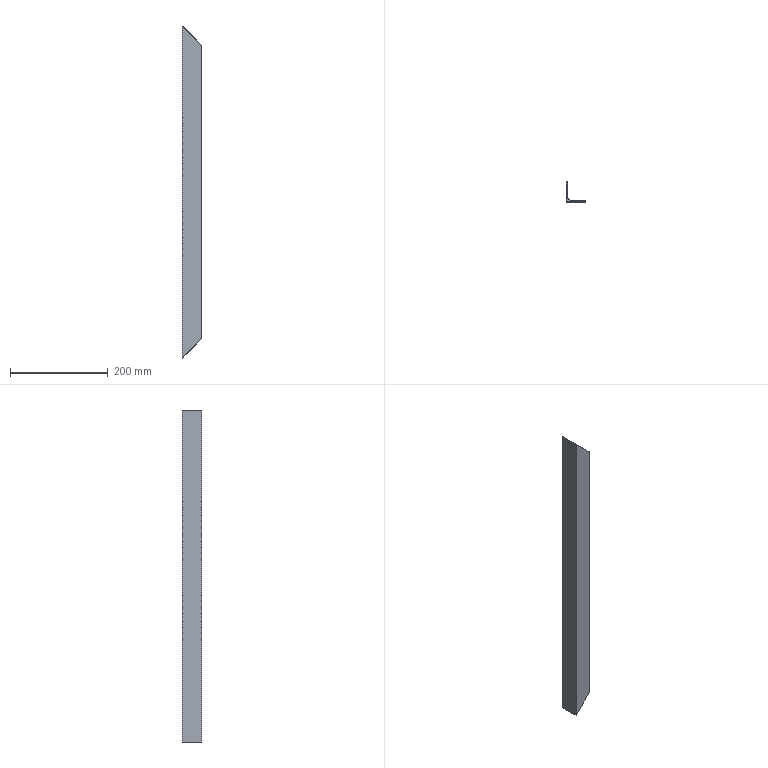Part | SolidWorks | features BaseBody 1 | 1 solid | 11 faces | box 40 x 40 x 680 mm | volume 155277 mm3 | plane 8 | cylinder 3 | commonest cylinder face diameters 2 x2 10 x1
STEP:
#1=CARTESIAN_POINT('',(-10.9,50.9,0.));
#2=VERTEX_POINT('',#1);
#3=CARTESIAN_POINT('',(-10.9,10.9,0.));
#4=VERTEX_POINT('',#3);
#5=CARTESIAN_POINT('',(-10.9,10.9,0.));
#6=DIRECTION('',(0.,-1.,0.));
#7=VECTOR('',#6,1000.);
#8=LINE('',#5,#7);
#9=EDGE_CURVE('',#2,#4,#8,.T.);
#10=ORIENTED_EDGE('',*,*,#9,.T.);
#11=CARTESIAN_POINT('',(-10.9,10.9,680.));
#12=VERTEX_POINT('',#11);
#13=CARTESIAN_POINT('',(-10.9,10.9,0.));
#14=DIRECTION('',(0.,0.,1.));
#15=VECTOR('',#14,1000.);
#16=LINE('',#13,#15);
#17=EDGE_CURVE('',#4,#12,#16,.T.);
#18=ORIENTED_EDGE('',*,*,#17,.T.);
#19=CARTESIAN_POINT('',(-10.9,50.9,680.));
#20=VERTEX_POINT('',#19);
#21=CARTESIAN_POINT('',(-10.9,10.9,680.));
#22=DIRECTION('',(0.,1.,0.));
#23=VECTOR('',#22,1000.);
#24=LINE('',#21,#23);
#25=EDGE_CURVE('',#12,#20,#24,.T.);
#26=ORIENTED_EDGE('',*,*,#25,.T.);
#27=CARTESIAN_POINT('',(-10.9,50.9,0.));
#28=DIRECTION('',(0.,0.,-1.));
#29=VECTOR('',#28,1000.);
#30=LINE('',#27,#29);
#31=EDGE_CURVE('',#20,#2,#30,.T.);
#32=ORIENTED_EDGE('',*,*,#31,.T.);
#33=EDGE_LOOP('',(#10,#18,#26,#32));
#34=FACE_OUTER_BOUND('',#33,.T.);
#35=CARTESIAN_POINT('',(-10.9,10.9,0.));
#36=DIRECTION('',(-1.,0.,0.));
#37=DIRECTION('',(0.,-1.,0.));
#38=AXIS2_PLACEMENT_3D('',#35,#36,#37);
#39=PLANE('',#38);
#40=ADVANCED_FACE('',(#34),#39,.T.);
#41=CARTESIAN_POINT('',(29.1,10.9,640.));
#42=VERTEX_POINT('',#41);
#43=CARTESIAN_POINT('',(29.1,10.9,640.));
#44=DIRECTION('',(-0.7071,0.,0.7071));
#45=VECTOR('',#44,1000.);
#46=LINE('',#43,#45);
#47=EDGE_CURVE('',#42,#12,#46,.T.);
#48=ORIENTED_EDGE('',*,*,#47,.T.);
#49=ORIENTED_EDGE('',*,*,#17,.F.);
#50=CARTESIAN_POINT('',(29.1,10.9,40.));
#51=VERTEX_POINT('',#50);
#52=CARTESIAN_POINT('',(-10.9,10.9,0.));
#53=DIRECTION('',(0.7071,0.,0.7071));
#54=VECTOR('',#53,1000.);
#55=LINE('',#52,#54);
#56=EDGE_CURVE('',#4,#51,#55,.T.);
#57=ORIENTED_EDGE('',*,*,#56,.T.);
#58=CARTESIAN_POINT('',(29.1,10.9,0.));
#59=DIRECTION('',(0.,0.,1.));
#60=VECTOR('',#59,1000.);
#61=LINE('',#58,#60);
#62=EDGE_CURVE('',#51,#42,#61,.T.);
#63=ORIENTED_EDGE('',*,*,#62,.T.);
#64=EDGE_LOOP('',(#48,#49,#57,#63));
#65=FACE_OUTER_BOUND('',#64,.T.);
#66=CARTESIAN_POINT('',(29.1,10.9,0.));
#67=DIRECTION('',(0.,-1.,0.));
#68=DIRECTION('',(1.,0.,0.));
#69=AXIS2_PLACEMENT_3D('',#66,#67,#68);
#70=PLANE('',#69);
#71=ADVANCED_FACE('',(#65),#70,.T.);
#72=CARTESIAN_POINT('',(29.1,12.9,40.));
#73=VERTEX_POINT('',#72);
#74=CARTESIAN_POINT('',(29.1,10.9,40.));
#75=DIRECTION('',(0.,1.,0.));
#76=VECTOR('',#75,1000.);
#77=LINE('',#74,#76);
#78=EDGE_CURVE('',#51,#73,#77,.T.);
#79=ORIENTED_EDGE('',*,*,#78,.F.);
#80=ORIENTED_EDGE('',*,*,#56,.F.);
#81=ORIENTED_EDGE('',*,*,#9,.F.);
#82=CARTESIAN_POINT('',(-8.9,50.9,2.));
#83=VERTEX_POINT('',#82);
#84=CARTESIAN_POINT('',(-10.9,50.9,0.));
#85=DIRECTION('',(-0.7071,0.,-0.7071));
#86=VECTOR('',#85,1000.);
#87=LINE('',#84,#86);
#88=EDGE_CURVE('',#83,#2,#87,.T.);
#89=ORIENTED_EDGE('',*,*,#88,.F.);
#90=CARTESIAN_POINT('',(-7.9,49.9,3.));
#91=VERTEX_POINT('',#90);
#92=CARTESIAN_POINT('',(-7.9,49.9,3.));
#93=CARTESIAN_POINT('',(-7.9,50.486,3.));
#94=CARTESIAN_POINT('',(-8.314,50.9,2.586));
#95=CARTESIAN_POINT('',(-8.9,50.9,2.));
#96=(BOUNDED_CURVE()B_SPLINE_CURVE(3,(#92,#93,#94,#95),.UNSPECIFIED.,.F.,.F.)B_SPLINE_CURVE_WITH_KNOTS((4,4),(0.,1.571),.UNSPECIFIED.)CURVE()GEOMETRIC_REPRESENTATION_ITEM()RATIONAL_B_SPLINE_CURVE((1.,0.8047,0.8047,1.))REPRESENTATION_ITEM(''));
#97=EDGE_CURVE('',#91,#83,#96,.T.);
#98=ORIENTED_EDGE('',*,*,#97,.F.);
#99=CARTESIAN_POINT('',(-7.9,18.9,3.));
#100=VERTEX_POINT('',#99);
#101=CARTESIAN_POINT('',(-7.9,10.9,3.));
#102=DIRECTION('',(0.,1.,0.));
#103=VECTOR('',#102,1000.);
#104=LINE('',#101,#103);
#105=EDGE_CURVE('',#100,#91,#104,.T.);
#106=ORIENTED_EDGE('',*,*,#105,.F.);
#107=CARTESIAN_POINT('',(-2.9,13.9,8.));
#108=VERTEX_POINT('',#107);
#109=CARTESIAN_POINT('',(-2.9,13.9,8.));
#110=CARTESIAN_POINT('',(-5.829,13.9,5.071));
#111=CARTESIAN_POINT('',(-7.9,15.971,3.));
#112=CARTESIAN_POINT('',(-7.9,18.9,3.));
#113=(BOUNDED_CURVE()B_SPLINE_CURVE(3,(#109,#110,#111,#112),.UNSPECIFIED.,.F.,.F.)B_SPLINE_CURVE_WITH_KNOTS((4,4),(1.571,3.142),.UNSPECIFIED.)CURVE()GEOMETRIC_REPRESENTATION_ITEM()RATIONAL_B_SPLINE_CURVE((1.,0.8047,0.8047,1.))REPRESENTATION_ITEM(''));
#114=EDGE_CURVE('',#108,#100,#113,.T.);
#115=ORIENTED_EDGE('',*,*,#114,.F.);
#116=CARTESIAN_POINT('',(28.1,13.9,39.));
#117=VERTEX_POINT('',#116);
#118=CARTESIAN_POINT('',(-10.9,13.9,0.));
#119=DIRECTION('',(-0.7071,0.,-0.7071));
#120=VECTOR('',#119,1000.);
#121=LINE('',#118,#120);
#122=EDGE_CURVE('',#117,#108,#121,.T.);
#123=ORIENTED_EDGE('',*,*,#122,.F.);
#124=CARTESIAN_POINT('',(29.1,12.9,40.));
#125=CARTESIAN_POINT('',(29.1,13.486,40.));
#126=CARTESIAN_POINT('',(28.686,13.9,39.586));
#127=CARTESIAN_POINT('',(28.1,13.9,39.));
#128=(BOUNDED_CURVE()B_SPLINE_CURVE(3,(#124,#125,#126,#127),.UNSPECIFIED.,.F.,.F.)B_SPLINE_CURVE_WITH_KNOTS((4,4),(0.,1.571),.UNSPECIFIED.)CURVE()GEOMETRIC_REPRESENTATION_ITEM()RATIONAL_B_SPLINE_CURVE((1.,0.8047,0.8047,1.))REPRESENTATION_ITEM(''));
#129=EDGE_CURVE('',#73,#117,#128,.T.);
#130=ORIENTED_EDGE('',*,*,#129,.F.);
#131=EDGE_LOOP('',(#79,#80,#81,#89,#98,#106,#115,#123,#130));
#132=FACE_OUTER_BOUND('',#131,.T.);
#133=CARTESIAN_POINT('',(-10.9,10.9,0.));
#134=DIRECTION('',(-0.7071,0.,0.7071));
#135=DIRECTION('',(0.7071,0.,0.7071));
#136=AXIS2_PLACEMENT_3D('',#133,#134,#135);
#137=PLANE('',#136);
#138=ADVANCED_FACE('',(#132),#137,.F.);
#139=CARTESIAN_POINT('',(-8.9,50.9,678.));
#140=VERTEX_POINT('',#139);
#141=CARTESIAN_POINT('',(-10.9,50.9,680.));
#142=DIRECTION('',(0.7071,0.,-0.7071));
#143=VECTOR('',#142,1000.);
#144=LINE('',#141,#143);
#145=EDGE_CURVE('',#20,#140,#144,.T.);
#146=ORIENTED_EDGE('',*,*,#145,.T.);
#147=CARTESIAN_POINT('',(-8.9,50.9,0.));
#148=DIRECTION('',(0.,0.,-1.));
#149=VECTOR('',#148,1000.);
#150=LINE('',#147,#149);
#151=EDGE_CURVE('',#140,#83,#150,.T.);
#152=ORIENTED_EDGE('',*,*,#151,.T.);
#153=ORIENTED_EDGE('',*,*,#88,.T.);
#154=ORIENTED_EDGE('',*,*,#31,.F.);
#155=EDGE_LOOP('',(#146,#152,#153,#154));
#156=FACE_OUTER_BOUND('',#155,.T.);
#157=CARTESIAN_POINT('',(-10.9,50.9,0.));
#158=DIRECTION('',(0.,1.,0.));
#159=DIRECTION('',(-1.,0.,0.));
#160=AXIS2_PLACEMENT_3D('',#157,#158,#159);
#161=PLANE('',#160);
#162=ADVANCED_FACE('',(#156),#161,.T.);
#163=CARTESIAN_POINT('',(-7.9,18.9,677.));
#164=VERTEX_POINT('',#163);
#165=CARTESIAN_POINT('',(-2.9,13.9,672.));
#166=VERTEX_POINT('',#165);
#167=CARTESIAN_POINT('',(-7.9,18.9,677.));
#168=CARTESIAN_POINT('',(-7.9,15.971,677.));
#169=CARTESIAN_POINT('',(-5.829,13.9,674.929));
#170=CARTESIAN_POINT('',(-2.9,13.9,672.));
#171=(BOUNDED_CURVE()B_SPLINE_CURVE(3,(#167,#168,#169,#170),.UNSPECIFIED.,.F.,.F.)B_SPLINE_CURVE_WITH_KNOTS((4,4),(0.,1.571),.UNSPECIFIED.)CURVE()GEOMETRIC_REPRESENTATION_ITEM()RATIONAL_B_SPLINE_CURVE((1.,0.8047,0.8047,1.))REPRESENTATION_ITEM(''));
#172=EDGE_CURVE('',#164,#166,#171,.T.);
#173=ORIENTED_EDGE('',*,*,#172,.F.);
#174=CARTESIAN_POINT('',(-7.9,49.9,677.));
#175=VERTEX_POINT('',#174);
#176=CARTESIAN_POINT('',(-7.9,0.,677.));
#177=DIRECTION('',(0.,-1.,0.));
#178=VECTOR('',#177,1000.);
#179=LINE('',#176,#178);
#180=EDGE_CURVE('',#175,#164,#179,.T.);
#181=ORIENTED_EDGE('',*,*,#180,.F.);
#182=CARTESIAN_POINT('',(-8.9,50.9,678.));
#183=CARTESIAN_POINT('',(-8.314,50.9,677.414));
#184=CARTESIAN_POINT('',(-7.9,50.486,677.));
#185=CARTESIAN_POINT('',(-7.9,49.9,677.));
#186=(BOUNDED_CURVE()B_SPLINE_CURVE(3,(#182,#183,#184,#185),.UNSPECIFIED.,.F.,.F.)B_SPLINE_CURVE_WITH_KNOTS((4,4),(1.571,3.142),.UNSPECIFIED.)CURVE()GEOMETRIC_REPRESENTATION_ITEM()RATIONAL_B_SPLINE_CURVE((1.,0.8047,0.8047,1.))REPRESENTATION_ITEM(''));
#187=EDGE_CURVE('',#140,#175,#186,.T.);
#188=ORIENTED_EDGE('',*,*,#187,.F.);
#189=ORIENTED_EDGE('',*,*,#145,.F.);
#190=ORIENTED_EDGE('',*,*,#25,.F.);
#191=ORIENTED_EDGE('',*,*,#47,.F.);
#192=CARTESIAN_POINT('',(29.1,12.9,640.));
#193=VERTEX_POINT('',#192);
#194=CARTESIAN_POINT('',(29.1,0.,640.));
#195=DIRECTION('',(0.,-1.,0.));
#196=VECTOR('',#195,1000.);
#197=LINE('',#194,#196);
#198=EDGE_CURVE('',#193,#42,#197,.T.);
#199=ORIENTED_EDGE('',*,*,#198,.F.);
#200=CARTESIAN_POINT('',(28.1,13.9,641.));
#201=VERTEX_POINT('',#200);
#202=CARTESIAN_POINT('',(28.1,13.9,641.));
#203=CARTESIAN_POINT('',(28.686,13.9,640.414));
#204=CARTESIAN_POINT('',(29.1,13.486,640.));
#205=CARTESIAN_POINT('',(29.1,12.9,640.));
#206=(BOUNDED_CURVE()B_SPLINE_CURVE(3,(#202,#203,#204,#205),.UNSPECIFIED.,.F.,.F.)B_SPLINE_CURVE_WITH_KNOTS((4,4),(1.571,3.142),.UNSPECIFIED.)CURVE()GEOMETRIC_REPRESENTATION_ITEM()RATIONAL_B_SPLINE_CURVE((1.,0.8047,0.8047,1.))REPRESENTATION_ITEM(''));
#207=EDGE_CURVE('',#201,#193,#206,.T.);
#208=ORIENTED_EDGE('',*,*,#207,.F.);
#209=CARTESIAN_POINT('',(334.55,13.9,334.55));
#210=DIRECTION('',(0.7071,0.,-0.7071));
#211=VECTOR('',#210,1000.);
#212=LINE('',#209,#211);
#213=EDGE_CURVE('',#166,#201,#212,.T.);
#214=ORIENTED_EDGE('',*,*,#213,.F.);
#215=EDGE_LOOP('',(#173,#181,#188,#189,#190,#191,#199,#208,#214));
#216=FACE_OUTER_BOUND('',#215,.T.);
#217=CARTESIAN_POINT('',(334.55,0.,334.55));
#218=DIRECTION('',(-0.7071,0.,-0.7071));
#219=DIRECTION('',(-0.7071,0.,0.7071));
#220=AXIS2_PLACEMENT_3D('',#217,#218,#219);
#221=PLANE('',#220);
#222=ADVANCED_FACE('',(#216),#221,.F.);
#223=ORIENTED_EDGE('',*,*,#198,.T.);
#224=ORIENTED_EDGE('',*,*,#62,.F.);
#225=ORIENTED_EDGE('',*,*,#78,.T.);
#226=CARTESIAN_POINT('',(29.1,12.9,0.));
#227=DIRECTION('',(0.,0.,1.));
#228=VECTOR('',#227,1000.);
#229=LINE('',#226,#228);
#230=EDGE_CURVE('',#73,#193,#229,.T.);
#231=ORIENTED_EDGE('',*,*,#230,.T.);
#232=EDGE_LOOP('',(#223,#224,#225,#231));
#233=FACE_OUTER_BOUND('',#232,.T.);
#234=CARTESIAN_POINT('',(29.1,12.9,0.));
#235=DIRECTION('',(1.,0.,0.));
#236=DIRECTION('',(0.,1.,0.));
#237=AXIS2_PLACEMENT_3D('',#234,#235,#236);
#238=PLANE('',#237);
#239=ADVANCED_FACE('',(#233),#238,.T.);
#240=ORIENTED_EDGE('',*,*,#207,.T.);
#241=ORIENTED_EDGE('',*,*,#230,.F.);
#242=ORIENTED_EDGE('',*,*,#129,.T.);
#243=CARTESIAN_POINT('',(28.1,13.9,0.));
#244=DIRECTION('',(0.,0.,1.));
#245=VECTOR('',#244,1000.);
#246=LINE('',#243,#245);
#247=EDGE_CURVE('',#117,#201,#246,.T.);
#248=ORIENTED_EDGE('',*,*,#247,.T.);
#249=EDGE_LOOP('',(#240,#241,#242,#248));
#250=FACE_OUTER_BOUND('',#249,.T.);
#251=CARTESIAN_POINT('',(28.1,12.9,0.));
#252=DIRECTION('',(0.,0.,1.));
#253=DIRECTION('',(1.,0.,0.));
#254=AXIS2_PLACEMENT_3D('',#251,#252,#253);
#255=CYLINDRICAL_SURFACE('',#254,1.);
#256=ADVANCED_FACE('',(#250),#255,.T.);
#257=ORIENTED_EDGE('',*,*,#187,.T.);
#258=CARTESIAN_POINT('',(-7.9,49.9,0.));
#259=DIRECTION('',(0.,0.,-1.));
#260=VECTOR('',#259,1000.);
#261=LINE('',#258,#260);
#262=EDGE_CURVE('',#175,#91,#261,.T.);
#263=ORIENTED_EDGE('',*,*,#262,.T.);
#264=ORIENTED_EDGE('',*,*,#97,.T.);
#265=ORIENTED_EDGE('',*,*,#151,.F.);
#266=EDGE_LOOP('',(#257,#263,#264,#265));
#267=FACE_OUTER_BOUND('',#266,.T.);
#268=CARTESIAN_POINT('',(-8.9,49.9,0.));
#269=DIRECTION('',(0.,0.,1.));
#270=DIRECTION('',(1.,0.,0.));
#271=AXIS2_PLACEMENT_3D('',#268,#269,#270);
#272=CYLINDRICAL_SURFACE('',#271,1.);
#273=ADVANCED_FACE('',(#267),#272,.T.);
#274=ORIENTED_EDGE('',*,*,#180,.T.);
#275=CARTESIAN_POINT('',(-7.9,18.9,0.));
#276=DIRECTION('',(0.,0.,-1.));
#277=VECTOR('',#276,1000.);
#278=LINE('',#275,#277);
#279=EDGE_CURVE('',#164,#100,#278,.T.);
#280=ORIENTED_EDGE('',*,*,#279,.T.);
#281=ORIENTED_EDGE('',*,*,#105,.T.);
#282=ORIENTED_EDGE('',*,*,#262,.F.);
#283=EDGE_LOOP('',(#274,#280,#281,#282));
#284=FACE_OUTER_BOUND('',#283,.T.);
#285=CARTESIAN_POINT('',(-7.9,49.9,0.));
#286=DIRECTION('',(1.,0.,0.));
#287=DIRECTION('',(0.,1.,0.));
#288=AXIS2_PLACEMENT_3D('',#285,#286,#287);
#289=PLANE('',#288);
#290=ADVANCED_FACE('',(#284),#289,.T.);
#291=ORIENTED_EDGE('',*,*,#279,.F.);
#292=ORIENTED_EDGE('',*,*,#172,.T.);
#293=CARTESIAN_POINT('',(-2.9,13.9,0.));
#294=DIRECTION('',(0.,0.,1.));
#295=VECTOR('',#294,1000.);
#296=LINE('',#293,#295);
#297=EDGE_CURVE('',#108,#166,#296,.T.);
#298=ORIENTED_EDGE('',*,*,#297,.F.);
#299=ORIENTED_EDGE('',*,*,#114,.T.);
#300=EDGE_LOOP('',(#291,#292,#298,#299));
#301=FACE_OUTER_BOUND('',#300,.T.);
#302=CARTESIAN_POINT('',(-2.9,18.9,0.));
#303=DIRECTION('',(0.,0.,1.));
#304=DIRECTION('',(1.,0.,0.));
#305=AXIS2_PLACEMENT_3D('',#302,#303,#304);
#306=CYLINDRICAL_SURFACE('',#305,5.);
#307=ADVANCED_FACE('',(#301),#306,.F.);
#308=ORIENTED_EDGE('',*,*,#213,.T.);
#309=ORIENTED_EDGE('',*,*,#247,.F.);
#310=ORIENTED_EDGE('',*,*,#122,.T.);
#311=ORIENTED_EDGE('',*,*,#297,.T.);
#312=EDGE_LOOP('',(#308,#309,#310,#311));
#313=FACE_OUTER_BOUND('',#312,.T.);
#314=CARTESIAN_POINT('',(-2.9,13.9,0.));
#315=DIRECTION('',(0.,1.,0.));
#316=DIRECTION('',(-1.,0.,0.));
#317=AXIS2_PLACEMENT_3D('',#314,#315,#316);
#318=PLANE('',#317);
#319=ADVANCED_FACE('',(#313),#318,.T.);
#320=CLOSED_SHELL('',(#40,#71,#138,#162,#222,#239,#256,#273,#290,#307,#319));
#321=MANIFOLD_SOLID_BREP('',#320);
#322=CARTESIAN_POINT('',(0.,0.,0.));
#323=DIRECTION('',(0.,0.,1.));
#324=DIRECTION('',(1.,0.,0.));
#325=AXIS2_PLACEMENT_3D('',#322,#323,#324);
#326=(LENGTH_UNIT()NAMED_UNIT(*)SI_UNIT(.MILLI.,.METRE.));
#327=UNCERTAINTY_MEASURE_WITH_UNIT(LENGTH_MEASURE(0.00001),#326,'','');
#328=(NAMED_UNIT(*)PLANE_ANGLE_UNIT()SI_UNIT($,.RADIAN.));
#329=(NAMED_UNIT(*)SI_UNIT($,.STERADIAN.)SOLID_ANGLE_UNIT());
#330=(GEOMETRIC_REPRESENTATION_CONTEXT(3)GLOBAL_UNCERTAINTY_ASSIGNED_CONTEXT((#327))GLOBAL_UNIT_ASSIGNED_CONTEXT((#326,#328,#329))REPRESENTATION_CONTEXT('',''));
#331=ADVANCED_BREP_SHAPE_REPRESENTATION('',(#321,#325),#330);